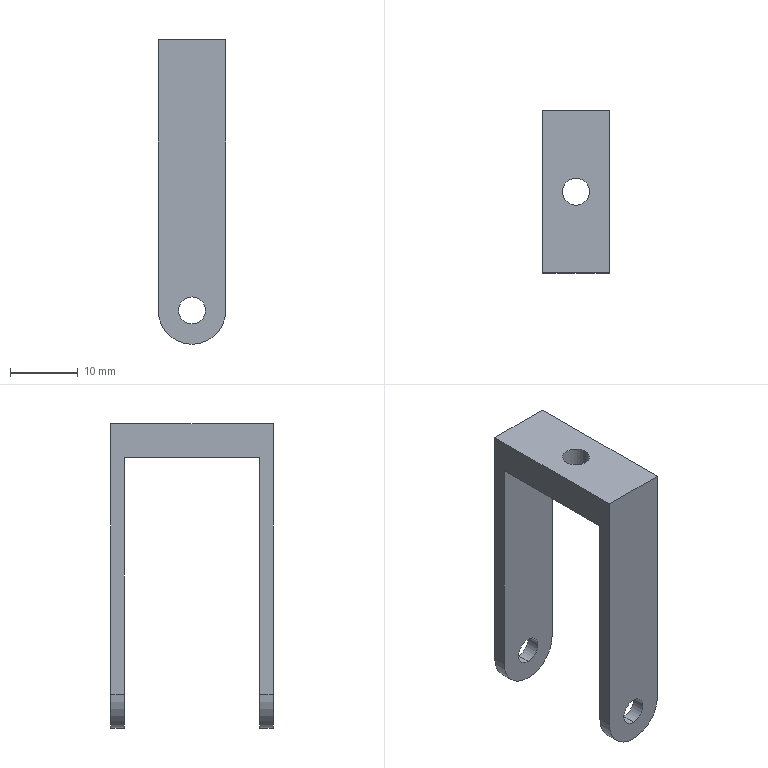Part | SolidWorks | features ICE 3, Extrusion 1 | 1 solid | 18 faces | box 10 x 24 x 45 mm | volume 2644 mm3 | cylinder 10 | plane 8 | commonest cylinder face diameters 4 x6 10 x4
STEP:
#1=CARTESIAN_POINT('',(2.,12.,40.));
#2=VERTEX_POINT('',#1);
#3=CARTESIAN_POINT('',(-2.,12.,40.));
#4=VERTEX_POINT('',#3);
#5=CARTESIAN_POINT('',(0.,12.,40.));
#6=DIRECTION('',(0.,0.,-1.));
#7=DIRECTION('',(-1.,0.,0.));
#8=AXIS2_PLACEMENT_3D('',#5,#6,#7);
#9=CIRCLE('',#8,2.);
#10=EDGE_CURVE('',#2,#4,#9,.T.);
#11=ORIENTED_EDGE('',*,*,#10,.F.);
#12=CARTESIAN_POINT('',(2.,12.,35.));
#13=VERTEX_POINT('',#12);
#14=CARTESIAN_POINT('',(2.,12.,40.));
#15=DIRECTION('',(0.,0.,-1.));
#16=VECTOR('',#15,1000.);
#17=LINE('',#14,#16);
#18=EDGE_CURVE('',#2,#13,#17,.T.);
#19=ORIENTED_EDGE('',*,*,#18,.T.);
#20=CARTESIAN_POINT('',(-2.,12.,35.));
#21=VERTEX_POINT('',#20);
#22=CARTESIAN_POINT('',(0.,12.,35.));
#23=DIRECTION('',(0.,0.,-1.));
#24=DIRECTION('',(-1.,0.,0.));
#25=AXIS2_PLACEMENT_3D('',#22,#23,#24);
#26=CIRCLE('',#25,2.);
#27=EDGE_CURVE('',#13,#21,#26,.T.);
#28=ORIENTED_EDGE('',*,*,#27,.T.);
#29=CARTESIAN_POINT('',(-2.,12.,40.));
#30=DIRECTION('',(0.,0.,-1.));
#31=VECTOR('',#30,1000.);
#32=LINE('',#29,#31);
#33=EDGE_CURVE('',#4,#21,#32,.T.);
#34=ORIENTED_EDGE('',*,*,#33,.F.);
#35=EDGE_LOOP('',(#11,#19,#28,#34));
#36=FACE_OUTER_BOUND('',#35,.T.);
#37=CARTESIAN_POINT('',(0.,12.,40.));
#38=DIRECTION('',(0.,0.,-1.));
#39=DIRECTION('',(-1.,0.,0.));
#40=AXIS2_PLACEMENT_3D('',#37,#38,#39);
#41=CYLINDRICAL_SURFACE('',#40,2.);
#42=ADVANCED_FACE('',(#36),#41,.F.);
#43=CARTESIAN_POINT('',(0.,0.,-2.));
#44=VERTEX_POINT('',#43);
#45=CARTESIAN_POINT('',(0.,0.,2.));
#46=VERTEX_POINT('',#45);
#47=CARTESIAN_POINT('',(0.,0.,0.));
#48=DIRECTION('',(0.,1.,0.));
#49=DIRECTION('',(0.,0.,1.));
#50=AXIS2_PLACEMENT_3D('',#47,#48,#49);
#51=CIRCLE('',#50,2.);
#52=EDGE_CURVE('',#44,#46,#51,.T.);
#53=ORIENTED_EDGE('',*,*,#52,.F.);
#54=CARTESIAN_POINT('',(0.,2.,-2.));
#55=VERTEX_POINT('',#54);
#56=CARTESIAN_POINT('',(0.,0.,-2.));
#57=DIRECTION('',(0.,1.,0.));
#58=VECTOR('',#57,1000.);
#59=LINE('',#56,#58);
#60=EDGE_CURVE('',#44,#55,#59,.T.);
#61=ORIENTED_EDGE('',*,*,#60,.T.);
#62=CARTESIAN_POINT('',(0.,2.,2.));
#63=VERTEX_POINT('',#62);
#64=CARTESIAN_POINT('',(0.,2.,0.));
#65=DIRECTION('',(0.,1.,0.));
#66=DIRECTION('',(0.,0.,-1.));
#67=AXIS2_PLACEMENT_3D('',#64,#65,#66);
#68=CIRCLE('',#67,2.);
#69=EDGE_CURVE('',#55,#63,#68,.T.);
#70=ORIENTED_EDGE('',*,*,#69,.T.);
#71=CARTESIAN_POINT('',(0.,0.,2.));
#72=DIRECTION('',(0.,1.,0.));
#73=VECTOR('',#72,1000.);
#74=LINE('',#71,#73);
#75=EDGE_CURVE('',#46,#63,#74,.T.);
#76=ORIENTED_EDGE('',*,*,#75,.F.);
#77=EDGE_LOOP('',(#53,#61,#70,#76));
#78=FACE_OUTER_BOUND('',#77,.T.);
#79=CARTESIAN_POINT('',(0.,0.,0.));
#80=DIRECTION('',(0.,1.,0.));
#81=DIRECTION('',(0.,0.,1.));
#82=AXIS2_PLACEMENT_3D('',#79,#80,#81);
#83=CYLINDRICAL_SURFACE('',#82,2.);
#84=ADVANCED_FACE('',(#78),#83,.F.);
#85=CARTESIAN_POINT('',(-5.,2.,0.));
#86=VERTEX_POINT('',#85);
#87=CARTESIAN_POINT('',(0.,2.,-5.));
#88=VERTEX_POINT('',#87);
#89=CARTESIAN_POINT('',(0.,2.,0.));
#90=DIRECTION('',(0.,-1.,0.));
#91=DIRECTION('',(0.,0.,-1.));
#92=AXIS2_PLACEMENT_3D('',#89,#90,#91);
#93=CIRCLE('',#92,5.);
#94=EDGE_CURVE('',#86,#88,#93,.T.);
#95=ORIENTED_EDGE('',*,*,#94,.T.);
#96=CARTESIAN_POINT('',(0.,0.,-5.));
#97=VERTEX_POINT('',#96);
#98=CARTESIAN_POINT('',(0.,24.,-5.));
#99=DIRECTION('',(0.,-1.,0.));
#100=VECTOR('',#99,1000.);
#101=LINE('',#98,#100);
#102=EDGE_CURVE('',#88,#97,#101,.T.);
#103=ORIENTED_EDGE('',*,*,#102,.T.);
#104=CARTESIAN_POINT('',(-5.,0.,0.));
#105=VERTEX_POINT('',#104);
#106=CARTESIAN_POINT('',(0.,0.,0.));
#107=DIRECTION('',(0.,1.,0.));
#108=DIRECTION('',(0.,0.,1.));
#109=AXIS2_PLACEMENT_3D('',#106,#107,#108);
#110=CIRCLE('',#109,5.);
#111=EDGE_CURVE('',#97,#105,#110,.T.);
#112=ORIENTED_EDGE('',*,*,#111,.T.);
#113=CARTESIAN_POINT('',(-5.,24.,0.));
#114=DIRECTION('',(0.,-1.,0.));
#115=VECTOR('',#114,1000.);
#116=LINE('',#113,#115);
#117=EDGE_CURVE('',#86,#105,#116,.T.);
#118=ORIENTED_EDGE('',*,*,#117,.F.);
#119=EDGE_LOOP('',(#95,#103,#112,#118));
#120=FACE_OUTER_BOUND('',#119,.T.);
#121=CARTESIAN_POINT('',(0.,24.,0.));
#122=DIRECTION('',(0.,-1.,0.));
#123=DIRECTION('',(0.,0.,-1.));
#124=AXIS2_PLACEMENT_3D('',#121,#122,#123);
#125=CYLINDRICAL_SURFACE('',#124,5.);
#126=ADVANCED_FACE('',(#120),#125,.T.);
#127=CARTESIAN_POINT('',(0.,22.,2.));
#128=VERTEX_POINT('',#127);
#129=CARTESIAN_POINT('',(0.,22.,-2.));
#130=VERTEX_POINT('',#129);
#131=CARTESIAN_POINT('',(0.,22.,0.));
#132=DIRECTION('',(0.,-1.,0.));
#133=DIRECTION('',(0.,0.,1.));
#134=AXIS2_PLACEMENT_3D('',#131,#132,#133);
#135=CIRCLE('',#134,2.);
#136=EDGE_CURVE('',#128,#130,#135,.T.);
#137=ORIENTED_EDGE('',*,*,#136,.T.);
#138=CARTESIAN_POINT('',(0.,24.,-2.));
#139=VERTEX_POINT('',#138);
#140=CARTESIAN_POINT('',(0.,0.,-2.));
#141=DIRECTION('',(0.,1.,0.));
#142=VECTOR('',#141,1000.);
#143=LINE('',#140,#142);
#144=EDGE_CURVE('',#130,#139,#143,.T.);
#145=ORIENTED_EDGE('',*,*,#144,.T.);
#146=CARTESIAN_POINT('',(0.,24.,2.));
#147=VERTEX_POINT('',#146);
#148=CARTESIAN_POINT('',(0.,24.,0.));
#149=DIRECTION('',(0.,1.,0.));
#150=DIRECTION('',(0.,0.,1.));
#151=AXIS2_PLACEMENT_3D('',#148,#149,#150);
#152=CIRCLE('',#151,2.);
#153=EDGE_CURVE('',#139,#147,#152,.T.);
#154=ORIENTED_EDGE('',*,*,#153,.T.);
#155=CARTESIAN_POINT('',(0.,0.,2.));
#156=DIRECTION('',(0.,1.,0.));
#157=VECTOR('',#156,1000.);
#158=LINE('',#155,#157);
#159=EDGE_CURVE('',#128,#147,#158,.T.);
#160=ORIENTED_EDGE('',*,*,#159,.F.);
#161=EDGE_LOOP('',(#137,#145,#154,#160));
#162=FACE_OUTER_BOUND('',#161,.T.);
#163=CARTESIAN_POINT('',(0.,0.,0.));
#164=DIRECTION('',(0.,1.,0.));
#165=DIRECTION('',(0.,0.,1.));
#166=AXIS2_PLACEMENT_3D('',#163,#164,#165);
#167=CYLINDRICAL_SURFACE('',#166,2.);
#168=ADVANCED_FACE('',(#162),#167,.F.);
#169=CARTESIAN_POINT('',(0.,24.,-5.));
#170=VERTEX_POINT('',#169);
#171=CARTESIAN_POINT('',(-5.,24.,0.));
#172=VERTEX_POINT('',#171);
#173=CARTESIAN_POINT('',(0.,24.,0.));
#174=DIRECTION('',(0.,1.,0.));
#175=DIRECTION('',(0.,0.,1.));
#176=AXIS2_PLACEMENT_3D('',#173,#174,#175);
#177=CIRCLE('',#176,5.);
#178=EDGE_CURVE('',#170,#172,#177,.T.);
#179=ORIENTED_EDGE('',*,*,#178,.F.);
#180=CARTESIAN_POINT('',(0.,22.,-5.));
#181=VERTEX_POINT('',#180);
#182=CARTESIAN_POINT('',(0.,24.,-5.));
#183=DIRECTION('',(0.,-1.,0.));
#184=VECTOR('',#183,1000.);
#185=LINE('',#182,#184);
#186=EDGE_CURVE('',#170,#181,#185,.T.);
#187=ORIENTED_EDGE('',*,*,#186,.T.);
#188=CARTESIAN_POINT('',(-5.,22.,0.));
#189=VERTEX_POINT('',#188);
#190=CARTESIAN_POINT('',(0.,22.,0.));
#191=DIRECTION('',(0.,1.,0.));
#192=DIRECTION('',(0.,0.,1.));
#193=AXIS2_PLACEMENT_3D('',#190,#191,#192);
#194=CIRCLE('',#193,5.);
#195=EDGE_CURVE('',#181,#189,#194,.T.);
#196=ORIENTED_EDGE('',*,*,#195,.T.);
#197=CARTESIAN_POINT('',(-5.,24.,0.));
#198=DIRECTION('',(0.,-1.,0.));
#199=VECTOR('',#198,1000.);
#200=LINE('',#197,#199);
#201=EDGE_CURVE('',#172,#189,#200,.T.);
#202=ORIENTED_EDGE('',*,*,#201,.F.);
#203=EDGE_LOOP('',(#179,#187,#196,#202));
#204=FACE_OUTER_BOUND('',#203,.T.);
#205=CARTESIAN_POINT('',(0.,24.,0.));
#206=DIRECTION('',(0.,-1.,0.));
#207=DIRECTION('',(0.,0.,-1.));
#208=AXIS2_PLACEMENT_3D('',#205,#206,#207);
#209=CYLINDRICAL_SURFACE('',#208,5.);
#210=ADVANCED_FACE('',(#204),#209,.T.);
#211=ORIENTED_EDGE('',*,*,#186,.F.);
#212=CARTESIAN_POINT('',(5.,24.,0.));
#213=VERTEX_POINT('',#212);
#214=CARTESIAN_POINT('',(0.,24.,0.));
#215=DIRECTION('',(0.,1.,0.));
#216=DIRECTION('',(0.,0.,1.));
#217=AXIS2_PLACEMENT_3D('',#214,#215,#216);
#218=CIRCLE('',#217,5.);
#219=EDGE_CURVE('',#213,#170,#218,.T.);
#220=ORIENTED_EDGE('',*,*,#219,.F.);
#221=CARTESIAN_POINT('',(5.,22.,0.));
#222=VERTEX_POINT('',#221);
#223=CARTESIAN_POINT('',(5.,24.,0.));
#224=DIRECTION('',(0.,-1.,0.));
#225=VECTOR('',#224,1000.);
#226=LINE('',#223,#225);
#227=EDGE_CURVE('',#213,#222,#226,.T.);
#228=ORIENTED_EDGE('',*,*,#227,.T.);
#229=CARTESIAN_POINT('',(0.,22.,0.));
#230=DIRECTION('',(0.,1.,0.));
#231=DIRECTION('',(0.,0.,1.));
#232=AXIS2_PLACEMENT_3D('',#229,#230,#231);
#233=CIRCLE('',#232,5.);
#234=EDGE_CURVE('',#222,#181,#233,.T.);
#235=ORIENTED_EDGE('',*,*,#234,.T.);
#236=EDGE_LOOP('',(#211,#220,#228,#235));
#237=FACE_OUTER_BOUND('',#236,.T.);
#238=CARTESIAN_POINT('',(0.,24.,0.));
#239=DIRECTION('',(0.,-1.,0.));
#240=DIRECTION('',(0.,0.,-1.));
#241=AXIS2_PLACEMENT_3D('',#238,#239,#240);
#242=CYLINDRICAL_SURFACE('',#241,5.);
#243=ADVANCED_FACE('',(#237),#242,.T.);
#244=ORIENTED_EDGE('',*,*,#144,.F.);
#245=CARTESIAN_POINT('',(0.,22.,0.));
#246=DIRECTION('',(0.,-1.,0.));
#247=DIRECTION('',(0.,0.,1.));
#248=AXIS2_PLACEMENT_3D('',#245,#246,#247);
#249=CIRCLE('',#248,2.);
#250=EDGE_CURVE('',#130,#128,#249,.T.);
#251=ORIENTED_EDGE('',*,*,#250,.T.);
#252=ORIENTED_EDGE('',*,*,#159,.T.);
#253=CARTESIAN_POINT('',(0.,24.,0.));
#254=DIRECTION('',(0.,1.,0.));
#255=DIRECTION('',(0.,0.,1.));
#256=AXIS2_PLACEMENT_3D('',#253,#254,#255);
#257=CIRCLE('',#256,2.);
#258=EDGE_CURVE('',#147,#139,#257,.T.);
#259=ORIENTED_EDGE('',*,*,#258,.T.);
#260=EDGE_LOOP('',(#244,#251,#252,#259));
#261=FACE_OUTER_BOUND('',#260,.T.);
#262=CARTESIAN_POINT('',(0.,0.,0.));
#263=DIRECTION('',(0.,1.,0.));
#264=DIRECTION('',(0.,0.,1.));
#265=AXIS2_PLACEMENT_3D('',#262,#263,#264);
#266=CYLINDRICAL_SURFACE('',#265,2.);
#267=ADVANCED_FACE('',(#261),#266,.F.);
#268=ORIENTED_EDGE('',*,*,#102,.F.);
#269=CARTESIAN_POINT('',(5.,2.,0.));
#270=VERTEX_POINT('',#269);
#271=CARTESIAN_POINT('',(0.,2.,0.));
#272=DIRECTION('',(0.,-1.,0.));
#273=DIRECTION('',(0.,0.,-1.));
#274=AXIS2_PLACEMENT_3D('',#271,#272,#273);
#275=CIRCLE('',#274,5.);
#276=EDGE_CURVE('',#88,#270,#275,.T.);
#277=ORIENTED_EDGE('',*,*,#276,.T.);
#278=CARTESIAN_POINT('',(5.,0.,0.));
#279=VERTEX_POINT('',#278);
#280=CARTESIAN_POINT('',(5.,24.,0.));
#281=DIRECTION('',(0.,-1.,0.));
#282=VECTOR('',#281,1000.);
#283=LINE('',#280,#282);
#284=EDGE_CURVE('',#270,#279,#283,.T.);
#285=ORIENTED_EDGE('',*,*,#284,.T.);
#286=CARTESIAN_POINT('',(0.,0.,0.));
#287=DIRECTION('',(0.,1.,0.));
#288=DIRECTION('',(0.,0.,1.));
#289=AXIS2_PLACEMENT_3D('',#286,#287,#288);
#290=CIRCLE('',#289,5.);
#291=EDGE_CURVE('',#279,#97,#290,.T.);
#292=ORIENTED_EDGE('',*,*,#291,.T.);
#293=EDGE_LOOP('',(#268,#277,#285,#292));
#294=FACE_OUTER_BOUND('',#293,.T.);
#295=CARTESIAN_POINT('',(0.,24.,0.));
#296=DIRECTION('',(0.,-1.,0.));
#297=DIRECTION('',(0.,0.,-1.));
#298=AXIS2_PLACEMENT_3D('',#295,#296,#297);
#299=CYLINDRICAL_SURFACE('',#298,5.);
#300=ADVANCED_FACE('',(#294),#299,.T.);
#301=ORIENTED_EDGE('',*,*,#201,.T.);
#302=CARTESIAN_POINT('',(-5.,22.,35.));
#303=VERTEX_POINT('',#302);
#304=CARTESIAN_POINT('',(-5.,22.,35.));
#305=DIRECTION('',(0.,0.,1.));
#306=VECTOR('',#305,1000.);
#307=LINE('',#304,#306);
#308=EDGE_CURVE('',#189,#303,#307,.T.);
#309=ORIENTED_EDGE('',*,*,#308,.T.);
#310=CARTESIAN_POINT('',(-5.,2.,35.));
#311=VERTEX_POINT('',#310);
#312=CARTESIAN_POINT('',(-5.,2.,35.));
#313=DIRECTION('',(0.,-1.,0.));
#314=VECTOR('',#313,1000.);
#315=LINE('',#312,#314);
#316=EDGE_CURVE('',#303,#311,#315,.T.);
#317=ORIENTED_EDGE('',*,*,#316,.T.);
#318=CARTESIAN_POINT('',(-5.,2.,-5.));
#319=DIRECTION('',(0.,0.,-1.));
#320=VECTOR('',#319,1000.);
#321=LINE('',#318,#320);
#322=EDGE_CURVE('',#311,#86,#321,.T.);
#323=ORIENTED_EDGE('',*,*,#322,.T.);
#324=ORIENTED_EDGE('',*,*,#117,.T.);
#325=CARTESIAN_POINT('',(-5.,0.,40.));
#326=VERTEX_POINT('',#325);
#327=CARTESIAN_POINT('',(-5.,0.,0.));
#328=DIRECTION('',(0.,0.,1.));
#329=VECTOR('',#328,1000.);
#330=LINE('',#327,#329);
#331=EDGE_CURVE('',#105,#326,#330,.T.);
#332=ORIENTED_EDGE('',*,*,#331,.T.);
#333=CARTESIAN_POINT('',(-5.,24.,40.));
#334=VERTEX_POINT('',#333);
#335=CARTESIAN_POINT('',(-5.,24.,40.));
#336=DIRECTION('',(0.,-1.,0.));
#337=VECTOR('',#336,1000.);
#338=LINE('',#335,#337);
#339=EDGE_CURVE('',#334,#326,#338,.T.);
#340=ORIENTED_EDGE('',*,*,#339,.F.);
#341=CARTESIAN_POINT('',(-5.,24.,0.));
#342=DIRECTION('',(0.,0.,1.));
#343=VECTOR('',#342,1000.);
#344=LINE('',#341,#343);
#345=EDGE_CURVE('',#172,#334,#344,.T.);
#346=ORIENTED_EDGE('',*,*,#345,.F.);
#347=EDGE_LOOP('',(#301,#309,#317,#323,#324,#332,#340,#346));
#348=FACE_OUTER_BOUND('',#347,.T.);
#349=CARTESIAN_POINT('',(-5.,24.,0.));
#350=DIRECTION('',(1.,0.,0.));
#351=DIRECTION('',(0.,0.,-1.));
#352=AXIS2_PLACEMENT_3D('',#349,#350,#351);
#353=PLANE('',#352);
#354=ADVANCED_FACE('',(#348),#353,.F.);
#355=CARTESIAN_POINT('',(0.,12.,40.));
#356=DIRECTION('',(0.,0.,-1.));
#357=DIRECTION('',(-1.,0.,0.));
#358=AXIS2_PLACEMENT_3D('',#355,#356,#357);
#359=CIRCLE('',#358,2.);
#360=EDGE_CURVE('',#4,#2,#359,.T.);
#361=ORIENTED_EDGE('',*,*,#360,.T.);
#362=ORIENTED_EDGE('',*,*,#10,.T.);
#363=EDGE_LOOP('',(#361,#362));
#364=FACE_BOUND('',#363,.T.);
#365=CARTESIAN_POINT('',(5.,0.,40.));
#366=VERTEX_POINT('',#365);
#367=CARTESIAN_POINT('',(-5.,0.,40.));
#368=DIRECTION('',(1.,0.,0.));
#369=VECTOR('',#368,1000.);
#370=LINE('',#367,#369);
#371=EDGE_CURVE('',#326,#366,#370,.T.);
#372=ORIENTED_EDGE('',*,*,#371,.T.);
#373=CARTESIAN_POINT('',(5.,24.,40.));
#374=VERTEX_POINT('',#373);
#375=CARTESIAN_POINT('',(5.,24.,40.));
#376=DIRECTION('',(0.,-1.,0.));
#377=VECTOR('',#376,1000.);
#378=LINE('',#375,#377);
#379=EDGE_CURVE('',#374,#366,#378,.T.);
#380=ORIENTED_EDGE('',*,*,#379,.F.);
#381=CARTESIAN_POINT('',(-5.,24.,40.));
#382=DIRECTION('',(1.,0.,0.));
#383=VECTOR('',#382,1000.);
#384=LINE('',#381,#383);
#385=EDGE_CURVE('',#334,#374,#384,.T.);
#386=ORIENTED_EDGE('',*,*,#385,.F.);
#387=ORIENTED_EDGE('',*,*,#339,.T.);
#388=EDGE_LOOP('',(#372,#380,#386,#387));
#389=FACE_OUTER_BOUND('',#388,.T.);
#390=CARTESIAN_POINT('',(-5.,24.,40.));
#391=DIRECTION('',(0.,0.,-1.));
#392=DIRECTION('',(-1.,0.,0.));
#393=AXIS2_PLACEMENT_3D('',#390,#391,#392);
#394=PLANE('',#393);
#395=ADVANCED_FACE('',(#364,#389),#394,.F.);
#396=CARTESIAN_POINT('',(5.,22.,35.));
#397=VERTEX_POINT('',#396);
#398=CARTESIAN_POINT('',(5.,2.,35.));
#399=VERTEX_POINT('',#398);
#400=CARTESIAN_POINT('',(5.,2.,35.));
#401=DIRECTION('',(0.,-1.,0.));
#402=VECTOR('',#401,1000.);
#403=LINE('',#400,#402);
#404=EDGE_CURVE('',#397,#399,#403,.T.);
#405=ORIENTED_EDGE('',*,*,#404,.F.);
#406=CARTESIAN_POINT('',(5.,22.,35.));
#407=DIRECTION('',(0.,0.,1.));
#408=VECTOR('',#407,1000.);
#409=LINE('',#406,#408);
#410=EDGE_CURVE('',#222,#397,#409,.T.);
#411=ORIENTED_EDGE('',*,*,#410,.F.);
#412=ORIENTED_EDGE('',*,*,#227,.F.);
#413=CARTESIAN_POINT('',(5.,24.,0.));
#414=DIRECTION('',(0.,0.,-1.));
#415=VECTOR('',#414,1000.);
#416=LINE('',#413,#415);
#417=EDGE_CURVE('',#374,#213,#416,.T.);
#418=ORIENTED_EDGE('',*,*,#417,.F.);
#419=ORIENTED_EDGE('',*,*,#379,.T.);
#420=CARTESIAN_POINT('',(5.,0.,0.));
#421=DIRECTION('',(0.,0.,-1.));
#422=VECTOR('',#421,1000.);
#423=LINE('',#420,#422);
#424=EDGE_CURVE('',#366,#279,#423,.T.);
#425=ORIENTED_EDGE('',*,*,#424,.T.);
#426=ORIENTED_EDGE('',*,*,#284,.F.);
#427=CARTESIAN_POINT('',(5.,2.,-5.));
#428=DIRECTION('',(0.,0.,-1.));
#429=VECTOR('',#428,1000.);
#430=LINE('',#427,#429);
#431=EDGE_CURVE('',#399,#270,#430,.T.);
#432=ORIENTED_EDGE('',*,*,#431,.F.);
#433=EDGE_LOOP('',(#405,#411,#412,#418,#419,#425,#426,#432));
#434=FACE_OUTER_BOUND('',#433,.T.);
#435=CARTESIAN_POINT('',(5.,24.,0.));
#436=DIRECTION('',(-1.,0.,0.));
#437=DIRECTION('',(0.,0.,1.));
#438=AXIS2_PLACEMENT_3D('',#435,#436,#437);
#439=PLANE('',#438);
#440=ADVANCED_FACE('',(#434),#439,.F.);
#441=ORIENTED_EDGE('',*,*,#258,.F.);
#442=ORIENTED_EDGE('',*,*,#153,.F.);
#443=EDGE_LOOP('',(#441,#442));
#444=FACE_BOUND('',#443,.T.);
#445=ORIENTED_EDGE('',*,*,#219,.T.);
#446=ORIENTED_EDGE('',*,*,#178,.T.);
#447=ORIENTED_EDGE('',*,*,#345,.T.);
#448=ORIENTED_EDGE('',*,*,#385,.T.);
#449=ORIENTED_EDGE('',*,*,#417,.T.);
#450=EDGE_LOOP('',(#445,#446,#447,#448,#449));
#451=FACE_OUTER_BOUND('',#450,.T.);
#452=CARTESIAN_POINT('',(0.,24.,0.));
#453=DIRECTION('',(0.,1.,0.));
#454=DIRECTION('',(0.,0.,1.));
#455=AXIS2_PLACEMENT_3D('',#452,#453,#454);
#456=PLANE('',#455);
#457=ADVANCED_FACE('',(#444,#451),#456,.T.);
#458=CARTESIAN_POINT('',(0.,0.,0.));
#459=DIRECTION('',(0.,1.,0.));
#460=DIRECTION('',(0.,0.,1.));
#461=AXIS2_PLACEMENT_3D('',#458,#459,#460);
#462=CIRCLE('',#461,2.);
#463=EDGE_CURVE('',#46,#44,#462,.T.);
#464=ORIENTED_EDGE('',*,*,#463,.T.);
#465=ORIENTED_EDGE('',*,*,#52,.T.);
#466=EDGE_LOOP('',(#464,#465));
#467=FACE_BOUND('',#466,.T.);
#468=ORIENTED_EDGE('',*,*,#291,.F.);
#469=ORIENTED_EDGE('',*,*,#424,.F.);
#470=ORIENTED_EDGE('',*,*,#371,.F.);
#471=ORIENTED_EDGE('',*,*,#331,.F.);
#472=ORIENTED_EDGE('',*,*,#111,.F.);
#473=EDGE_LOOP('',(#468,#469,#470,#471,#472));
#474=FACE_OUTER_BOUND('',#473,.T.);
#475=CARTESIAN_POINT('',(0.,0.,0.));
#476=DIRECTION('',(0.,1.,0.));
#477=DIRECTION('',(0.,0.,1.));
#478=AXIS2_PLACEMENT_3D('',#475,#476,#477);
#479=PLANE('',#478);
#480=ADVANCED_FACE('',(#467,#474),#479,.F.);
#481=ORIENTED_EDGE('',*,*,#60,.F.);
#482=ORIENTED_EDGE('',*,*,#463,.F.);
#483=ORIENTED_EDGE('',*,*,#75,.T.);
#484=CARTESIAN_POINT('',(0.,2.,0.));
#485=DIRECTION('',(0.,1.,0.));
#486=DIRECTION('',(0.,0.,-1.));
#487=AXIS2_PLACEMENT_3D('',#484,#485,#486);
#488=CIRCLE('',#487,2.);
#489=EDGE_CURVE('',#63,#55,#488,.T.);
#490=ORIENTED_EDGE('',*,*,#489,.T.);
#491=EDGE_LOOP('',(#481,#482,#483,#490));
#492=FACE_OUTER_BOUND('',#491,.T.);
#493=CARTESIAN_POINT('',(0.,0.,0.));
#494=DIRECTION('',(0.,1.,0.));
#495=DIRECTION('',(0.,0.,1.));
#496=AXIS2_PLACEMENT_3D('',#493,#494,#495);
#497=CYLINDRICAL_SURFACE('',#496,2.);
#498=ADVANCED_FACE('',(#492),#497,.F.);
#499=ORIENTED_EDGE('',*,*,#136,.F.);
#500=ORIENTED_EDGE('',*,*,#250,.F.);
#501=EDGE_LOOP('',(#499,#500));
#502=FACE_BOUND('',#501,.T.);
#503=ORIENTED_EDGE('',*,*,#410,.T.);
#504=CARTESIAN_POINT('',(-5.,22.,35.));
#505=DIRECTION('',(1.,0.,0.));
#506=VECTOR('',#505,1000.);
#507=LINE('',#504,#506);
#508=EDGE_CURVE('',#303,#397,#507,.T.);
#509=ORIENTED_EDGE('',*,*,#508,.F.);
#510=ORIENTED_EDGE('',*,*,#308,.F.);
#511=ORIENTED_EDGE('',*,*,#195,.F.);
#512=ORIENTED_EDGE('',*,*,#234,.F.);
#513=EDGE_LOOP('',(#503,#509,#510,#511,#512));
#514=FACE_OUTER_BOUND('',#513,.T.);
#515=CARTESIAN_POINT('',(-5.,22.,35.));
#516=DIRECTION('',(0.,1.,0.));
#517=DIRECTION('',(0.,0.,1.));
#518=AXIS2_PLACEMENT_3D('',#515,#516,#517);
#519=PLANE('',#518);
#520=ADVANCED_FACE('',(#502,#514),#519,.F.);
#521=ORIENTED_EDGE('',*,*,#489,.F.);
#522=ORIENTED_EDGE('',*,*,#69,.F.);
#523=EDGE_LOOP('',(#521,#522));
#524=FACE_BOUND('',#523,.T.);
#525=ORIENTED_EDGE('',*,*,#94,.F.);
#526=ORIENTED_EDGE('',*,*,#322,.F.);
#527=CARTESIAN_POINT('',(-5.,2.,35.));
#528=DIRECTION('',(1.,0.,0.));
#529=VECTOR('',#528,1000.);
#530=LINE('',#527,#529);
#531=EDGE_CURVE('',#311,#399,#530,.T.);
#532=ORIENTED_EDGE('',*,*,#531,.T.);
#533=ORIENTED_EDGE('',*,*,#431,.T.);
#534=ORIENTED_EDGE('',*,*,#276,.F.);
#535=EDGE_LOOP('',(#525,#526,#532,#533,#534));
#536=FACE_OUTER_BOUND('',#535,.T.);
#537=CARTESIAN_POINT('',(-5.,2.,-5.));
#538=DIRECTION('',(0.,-1.,0.));
#539=DIRECTION('',(0.,0.,-1.));
#540=AXIS2_PLACEMENT_3D('',#537,#538,#539);
#541=PLANE('',#540);
#542=ADVANCED_FACE('',(#524,#536),#541,.F.);
#543=CARTESIAN_POINT('',(0.,12.,35.));
#544=DIRECTION('',(0.,0.,-1.));
#545=DIRECTION('',(-1.,0.,0.));
#546=AXIS2_PLACEMENT_3D('',#543,#544,#545);
#547=CIRCLE('',#546,2.);
#548=EDGE_CURVE('',#21,#13,#547,.T.);
#549=ORIENTED_EDGE('',*,*,#548,.F.);
#550=ORIENTED_EDGE('',*,*,#27,.F.);
#551=EDGE_LOOP('',(#549,#550));
#552=FACE_BOUND('',#551,.T.);
#553=ORIENTED_EDGE('',*,*,#404,.T.);
#554=ORIENTED_EDGE('',*,*,#531,.F.);
#555=ORIENTED_EDGE('',*,*,#316,.F.);
#556=ORIENTED_EDGE('',*,*,#508,.T.);
#557=EDGE_LOOP('',(#553,#554,#555,#556));
#558=FACE_OUTER_BOUND('',#557,.T.);
#559=CARTESIAN_POINT('',(-5.,2.,35.));
#560=DIRECTION('',(0.,0.,1.));
#561=DIRECTION('',(1.,0.,0.));
#562=AXIS2_PLACEMENT_3D('',#559,#560,#561);
#563=PLANE('',#562);
#564=ADVANCED_FACE('',(#552,#558),#563,.F.);
#565=ORIENTED_EDGE('',*,*,#18,.F.);
#566=ORIENTED_EDGE('',*,*,#360,.F.);
#567=ORIENTED_EDGE('',*,*,#33,.T.);
#568=ORIENTED_EDGE('',*,*,#548,.T.);
#569=EDGE_LOOP('',(#565,#566,#567,#568));
#570=FACE_OUTER_BOUND('',#569,.T.);
#571=CARTESIAN_POINT('',(0.,12.,40.));
#572=DIRECTION('',(0.,0.,-1.));
#573=DIRECTION('',(-1.,0.,0.));
#574=AXIS2_PLACEMENT_3D('',#571,#572,#573);
#575=CYLINDRICAL_SURFACE('',#574,2.);
#576=ADVANCED_FACE('',(#570),#575,.F.);
#577=CLOSED_SHELL('',(#42,#84,#126,#168,#210,#243,#267,#300,#354,#395,#440,#457,#480,#498,#520,#542,#564,#576));
#578=MANIFOLD_SOLID_BREP('',#577);
#579=CARTESIAN_POINT('',(0.,0.,0.));
#580=DIRECTION('',(0.,0.,1.));
#581=DIRECTION('',(1.,0.,0.));
#582=AXIS2_PLACEMENT_3D('',#579,#580,#581);
#583=(LENGTH_UNIT()NAMED_UNIT(*)SI_UNIT(.MILLI.,.METRE.));
#584=UNCERTAINTY_MEASURE_WITH_UNIT(LENGTH_MEASURE(0.00001),#583,'','');
#585=(NAMED_UNIT(*)PLANE_ANGLE_UNIT()SI_UNIT($,.RADIAN.));
#586=(NAMED_UNIT(*)SI_UNIT($,.STERADIAN.)SOLID_ANGLE_UNIT());
#587=(GEOMETRIC_REPRESENTATION_CONTEXT(3)GLOBAL_UNCERTAINTY_ASSIGNED_CONTEXT((#584))GLOBAL_UNIT_ASSIGNED_CONTEXT((#583,#585,#586))REPRESENTATION_CONTEXT('',''));
#588=ADVANCED_BREP_SHAPE_REPRESENTATION('',(#578,#582),#587);